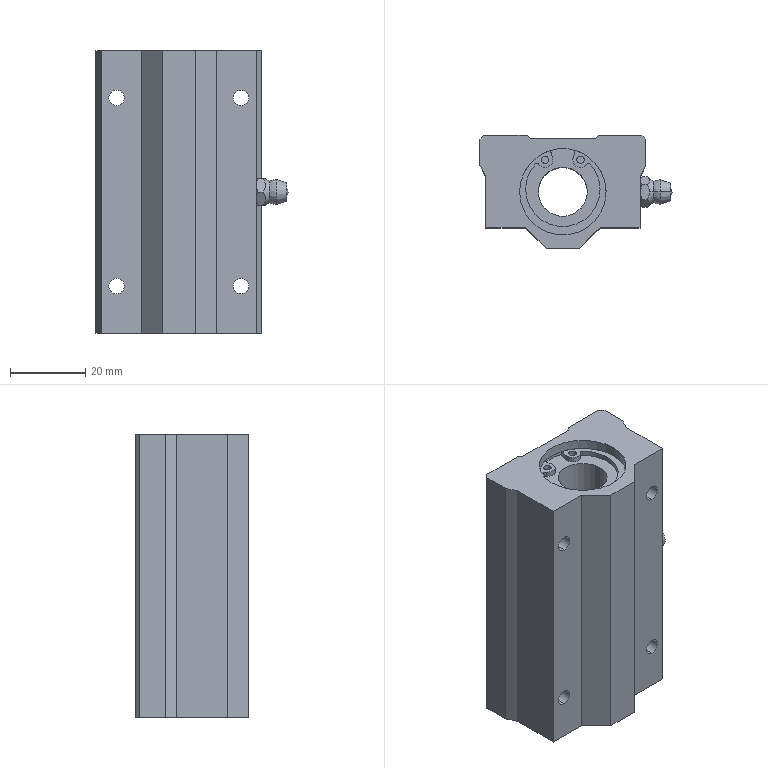Part | STEP file | 001-003-LMW56_d13 | 1 solid | 107 faces | box 51 x 30 x 75 mm | volume 69103 mm3 | cylinder 48 | plane 41 | cone 12 | other 4 | torus 2 | commonest cylinder face diameters 2 x8 4.134 x8 4.1 x6 19.77 x6 23.5 x6 1 x4